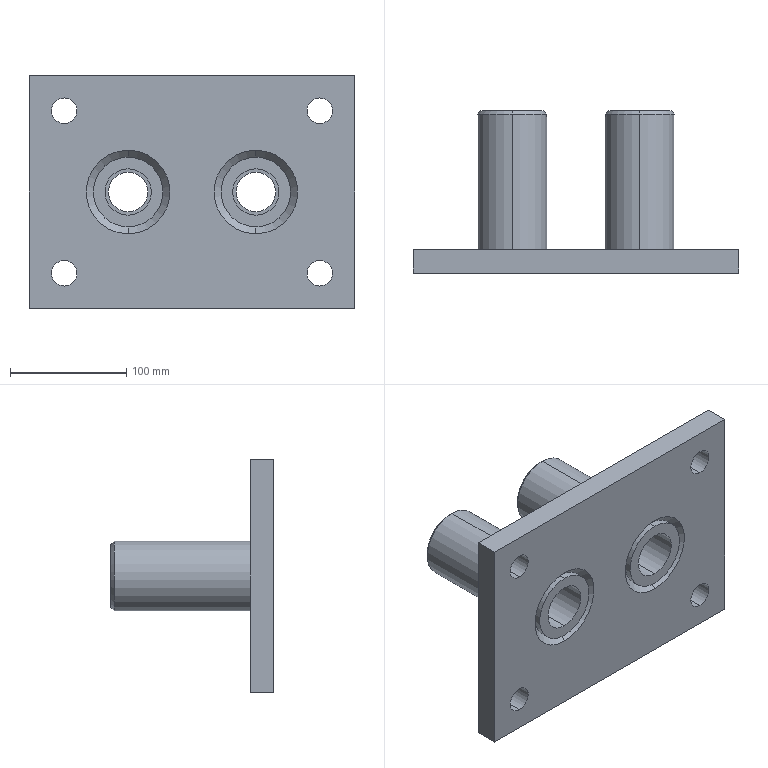Part | SolidWorks | features ICE 5, Chamfer 2, Extrusion 1, MirrorSolid 1 | 3 solids | 60 faces | box 280 x 140 x 200 mm | volume 1375614 mm3 | cylinder 32 | plane 16 | cone 12 | commonest cylinder face diameters 22 x8 60 x8 34 x4 40 x4 42.5 x4 50 x4